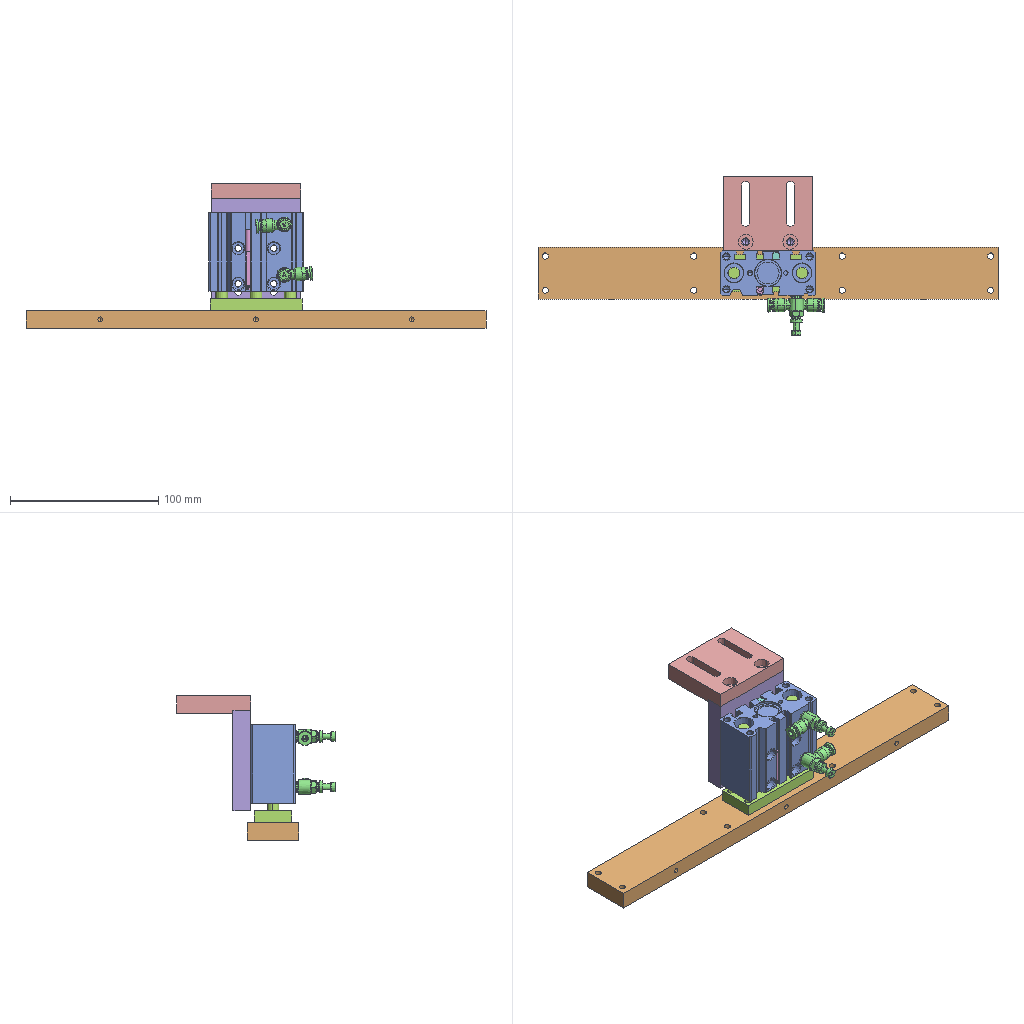Assembly | SolidWorks | 5 different items | 6 placed | box 310 x 107 x 98 mm
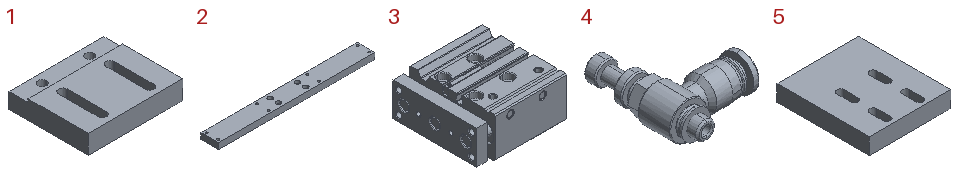Parts list (item | quantity | size | volume | features):
1 | x1 | 60 x 50 x 12 mm | 29704 mm3 | features Cut 1, Extrusion 1, HoleWzd 1, ICE 1
2 | x1 | 310 x 35 x 12 mm | 126366 mm3 | features HoleWzd 3, Extrusion 1, LPattern 1
3 | x1 | 66 x 64 x 30 mm | 89467 mm3 | features BaseBody 4
4 | x2 | 24 x 30 x 10 mm | 1863 mm3 | features BaseBody 1
5 | x1 | 60 x 67.5 x 12 mm | 44553 mm3 | features Cut 1, Extrusion 1, HoleWzd 1
Mates (type | each side: item.copy, entity, surface, feature):
Coincident | 3.1 face plane _TCL-16x20-0_20fp-1-solid1 | 2.1 face plane Boss-Extrude 1
Width | 3.1 face plane _TCL-16x20-0_20fp-1-solid1 | 3.1 face plane _TCL-16x20-0_20fp-1-solid1 | 2.1 face plane Boss-Extrude 1 | 2.1 face plane Boss-Extrude 1
Width | 2.1 face plane Boss-Extrude 1 | 2.1 face plane Boss-Extrude 1 | 3.1 face plane _TCL-16x20-0_20fp-1-solid1 | 3.1 face plane _TCL-16x20-0_20fp-1-solid1
Coincident | 3.1 face plane _TC-L-16x2020_b-1-solid1 | 5.1 face plane Boss-Extrude 1
Width | 5.1 face plane Boss-Extrude 1 | 5.1 face plane Boss-Extrude 1 | 3.1 face plane _TC-L-16x2020_b-1-solid1 | 3.1 face plane _TC-L-16x2020_b-1-solid1
DistanceDim | 3.1 face plane _TC-L-16x2020_b-1-solid1 | 5.1 face plane Boss-Extrude 1
Coincident | 5.1 face plane Boss-Extrude 1 | 1.1 face plane Cut-Extrude 1
Coincident | 5.1 face plane Boss-Extrude 1 | 1.1 face plane Boss-Extrude 1 | 2 times
Coincident | 1.1 plane | assembly plane | 3 times
Coincident | 4.1 face plane 输入1 | 4.2 face plane 输入1
Coincident | 3.1 face plane _TC-L-16x2020_b-1-solid1 | 4.2 face plane 输入1
Concentric | 3.1 face cylinder _TC-L-16x2020_b-1-solid1 | 4.2 face cylinder 输入1
Concentric | 3.1 face cylinder _TC-L-16x2020_b-1-solid1 | 4.1 face cylinder 输入1